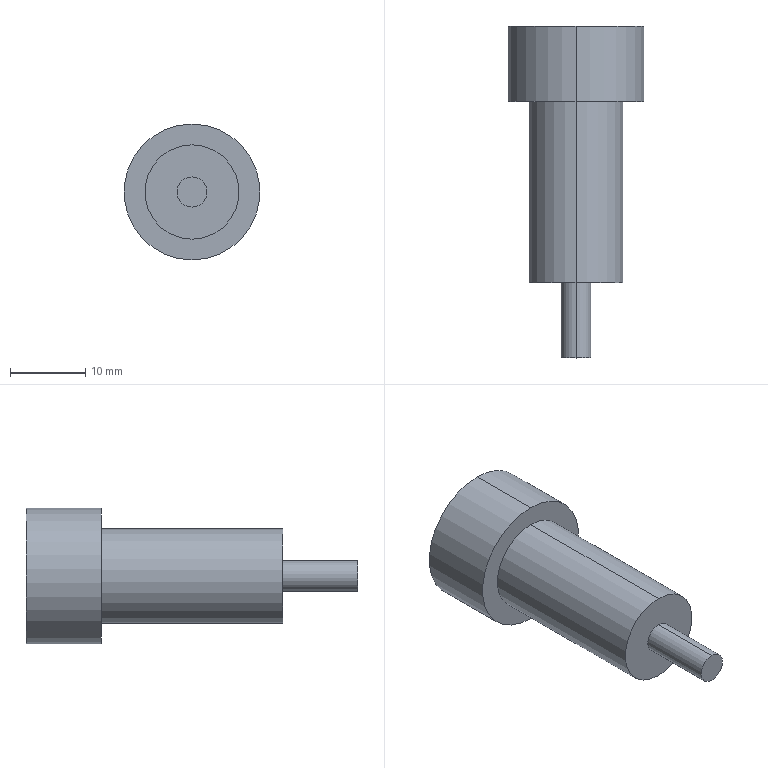Part | SolidWorks | features ICE 3, Extrusion 1 | 1 solid | 17 faces | box 18 x 44 x 18 mm | volume 5338 mm3 | plane 11 | cylinder 6 | commonest cylinder face diameters 4 x2 12.5 x2 18 x2
STEP:
#1=CARTESIAN_POINT('',(0.,44.,9.));
#2=VERTEX_POINT('',#1);
#3=CARTESIAN_POINT('',(0.,44.,-9.));
#4=VERTEX_POINT('',#3);
#5=CARTESIAN_POINT('',(0.,44.,0.));
#6=DIRECTION('',(0.,1.,0.));
#7=DIRECTION('',(0.,0.,1.));
#8=AXIS2_PLACEMENT_3D('',#5,#6,#7);
#9=CIRCLE('',#8,9.);
#10=EDGE_CURVE('',#2,#4,#9,.T.);
#11=ORIENTED_EDGE('',*,*,#10,.F.);
#12=CARTESIAN_POINT('',(0.,34.,9.));
#13=VERTEX_POINT('',#12);
#14=CARTESIAN_POINT('',(0.,44.,9.));
#15=DIRECTION('',(0.,-1.,0.));
#16=VECTOR('',#15,1000.);
#17=LINE('',#14,#16);
#18=EDGE_CURVE('',#2,#13,#17,.T.);
#19=ORIENTED_EDGE('',*,*,#18,.T.);
#20=CARTESIAN_POINT('',(0.,34.,-9.));
#21=VERTEX_POINT('',#20);
#22=CARTESIAN_POINT('',(0.,34.,0.));
#23=DIRECTION('',(0.,1.,0.));
#24=DIRECTION('',(0.,0.,1.));
#25=AXIS2_PLACEMENT_3D('',#22,#23,#24);
#26=CIRCLE('',#25,9.);
#27=EDGE_CURVE('',#13,#21,#26,.T.);
#28=ORIENTED_EDGE('',*,*,#27,.T.);
#29=CARTESIAN_POINT('',(0.,44.,-9.));
#30=DIRECTION('',(0.,-1.,0.));
#31=VECTOR('',#30,1000.);
#32=LINE('',#29,#31);
#33=EDGE_CURVE('',#4,#21,#32,.T.);
#34=ORIENTED_EDGE('',*,*,#33,.F.);
#35=EDGE_LOOP('',(#11,#19,#28,#34));
#36=FACE_OUTER_BOUND('',#35,.T.);
#37=CARTESIAN_POINT('',(0.,44.,0.));
#38=DIRECTION('',(0.,-1.,0.));
#39=DIRECTION('',(0.,0.,-1.));
#40=AXIS2_PLACEMENT_3D('',#37,#38,#39);
#41=CYLINDRICAL_SURFACE('',#40,9.);
#42=ADVANCED_FACE('',(#36),#41,.T.);
#43=CARTESIAN_POINT('',(0.,34.,6.25));
#44=VERTEX_POINT('',#43);
#45=CARTESIAN_POINT('',(0.,34.,-6.25));
#46=VERTEX_POINT('',#45);
#47=CARTESIAN_POINT('',(0.,34.,0.));
#48=DIRECTION('',(0.,1.,0.));
#49=DIRECTION('',(0.,0.,1.));
#50=AXIS2_PLACEMENT_3D('',#47,#48,#49);
#51=CIRCLE('',#50,6.25);
#52=EDGE_CURVE('',#44,#46,#51,.T.);
#53=ORIENTED_EDGE('',*,*,#52,.F.);
#54=CARTESIAN_POINT('',(0.,10.,6.25));
#55=VERTEX_POINT('',#54);
#56=CARTESIAN_POINT('',(0.,34.,6.25));
#57=DIRECTION('',(0.,-1.,0.));
#58=VECTOR('',#57,1000.);
#59=LINE('',#56,#58);
#60=EDGE_CURVE('',#44,#55,#59,.T.);
#61=ORIENTED_EDGE('',*,*,#60,.T.);
#62=CARTESIAN_POINT('',(0.,10.,-6.25));
#63=VERTEX_POINT('',#62);
#64=CARTESIAN_POINT('',(0.,10.,0.));
#65=DIRECTION('',(0.,1.,0.));
#66=DIRECTION('',(0.,0.,1.));
#67=AXIS2_PLACEMENT_3D('',#64,#65,#66);
#68=CIRCLE('',#67,6.25);
#69=EDGE_CURVE('',#55,#63,#68,.T.);
#70=ORIENTED_EDGE('',*,*,#69,.T.);
#71=CARTESIAN_POINT('',(0.,34.,-6.25));
#72=DIRECTION('',(0.,-1.,0.));
#73=VECTOR('',#72,1000.);
#74=LINE('',#71,#73);
#75=EDGE_CURVE('',#46,#63,#74,.T.);
#76=ORIENTED_EDGE('',*,*,#75,.F.);
#77=EDGE_LOOP('',(#53,#61,#70,#76));
#78=FACE_OUTER_BOUND('',#77,.T.);
#79=CARTESIAN_POINT('',(0.,34.,0.));
#80=DIRECTION('',(0.,-1.,0.));
#81=DIRECTION('',(0.,0.,-1.));
#82=AXIS2_PLACEMENT_3D('',#79,#80,#81);
#83=CYLINDRICAL_SURFACE('',#82,6.25);
#84=ADVANCED_FACE('',(#78),#83,.T.);
#85=CARTESIAN_POINT('',(0.,10.,2.));
#86=VERTEX_POINT('',#85);
#87=CARTESIAN_POINT('',(0.,10.,-2.));
#88=VERTEX_POINT('',#87);
#89=CARTESIAN_POINT('',(0.,10.,0.));
#90=DIRECTION('',(0.,1.,0.));
#91=DIRECTION('',(0.,0.,1.));
#92=AXIS2_PLACEMENT_3D('',#89,#90,#91);
#93=CIRCLE('',#92,2.);
#94=EDGE_CURVE('',#86,#88,#93,.T.);
#95=ORIENTED_EDGE('',*,*,#94,.F.);
#96=CARTESIAN_POINT('',(0.,0.,2.));
#97=VERTEX_POINT('',#96);
#98=CARTESIAN_POINT('',(0.,10.,2.));
#99=DIRECTION('',(0.,-1.,0.));
#100=VECTOR('',#99,1000.);
#101=LINE('',#98,#100);
#102=EDGE_CURVE('',#86,#97,#101,.T.);
#103=ORIENTED_EDGE('',*,*,#102,.T.);
#104=CARTESIAN_POINT('',(0.,0.,-2.));
#105=VERTEX_POINT('',#104);
#106=CARTESIAN_POINT('',(0.,0.,0.));
#107=DIRECTION('',(0.,1.,0.));
#108=DIRECTION('',(0.,0.,1.));
#109=AXIS2_PLACEMENT_3D('',#106,#107,#108);
#110=CIRCLE('',#109,2.);
#111=EDGE_CURVE('',#97,#105,#110,.T.);
#112=ORIENTED_EDGE('',*,*,#111,.T.);
#113=CARTESIAN_POINT('',(0.,10.,-2.));
#114=DIRECTION('',(0.,-1.,0.));
#115=VECTOR('',#114,1000.);
#116=LINE('',#113,#115);
#117=EDGE_CURVE('',#88,#105,#116,.T.);
#118=ORIENTED_EDGE('',*,*,#117,.F.);
#119=EDGE_LOOP('',(#95,#103,#112,#118));
#120=FACE_OUTER_BOUND('',#119,.T.);
#121=CARTESIAN_POINT('',(0.,10.,0.));
#122=DIRECTION('',(0.,-1.,0.));
#123=DIRECTION('',(0.,0.,-1.));
#124=AXIS2_PLACEMENT_3D('',#121,#122,#123);
#125=CYLINDRICAL_SURFACE('',#124,2.);
#126=ADVANCED_FACE('',(#120),#125,.T.);
#127=ORIENTED_EDGE('',*,*,#102,.F.);
#128=CARTESIAN_POINT('',(0.,10.,0.));
#129=DIRECTION('',(0.,1.,0.));
#130=DIRECTION('',(0.,0.,1.));
#131=AXIS2_PLACEMENT_3D('',#128,#129,#130);
#132=CIRCLE('',#131,2.);
#133=EDGE_CURVE('',#88,#86,#132,.T.);
#134=ORIENTED_EDGE('',*,*,#133,.F.);
#135=ORIENTED_EDGE('',*,*,#117,.T.);
#136=CARTESIAN_POINT('',(0.,0.,0.));
#137=DIRECTION('',(0.,1.,0.));
#138=DIRECTION('',(0.,0.,1.));
#139=AXIS2_PLACEMENT_3D('',#136,#137,#138);
#140=CIRCLE('',#139,2.);
#141=EDGE_CURVE('',#105,#97,#140,.T.);
#142=ORIENTED_EDGE('',*,*,#141,.T.);
#143=EDGE_LOOP('',(#127,#134,#135,#142));
#144=FACE_OUTER_BOUND('',#143,.T.);
#145=CARTESIAN_POINT('',(0.,10.,0.));
#146=DIRECTION('',(0.,-1.,0.));
#147=DIRECTION('',(0.,0.,-1.));
#148=AXIS2_PLACEMENT_3D('',#145,#146,#147);
#149=CYLINDRICAL_SURFACE('',#148,2.);
#150=ADVANCED_FACE('',(#144),#149,.T.);
#151=ORIENTED_EDGE('',*,*,#141,.F.);
#152=ORIENTED_EDGE('',*,*,#111,.F.);
#153=EDGE_LOOP('',(#151,#152));
#154=FACE_OUTER_BOUND('',#153,.T.);
#155=CARTESIAN_POINT('',(0.,0.,0.));
#156=DIRECTION('',(0.,1.,0.));
#157=DIRECTION('',(0.,0.,1.));
#158=AXIS2_PLACEMENT_3D('',#155,#156,#157);
#159=PLANE('',#158);
#160=ADVANCED_FACE('',(#154),#159,.F.);
#161=ORIENTED_EDGE('',*,*,#60,.F.);
#162=CARTESIAN_POINT('',(0.,34.,0.));
#163=DIRECTION('',(0.,1.,0.));
#164=DIRECTION('',(0.,0.,1.));
#165=AXIS2_PLACEMENT_3D('',#162,#163,#164);
#166=CIRCLE('',#165,6.25);
#167=EDGE_CURVE('',#46,#44,#166,.T.);
#168=ORIENTED_EDGE('',*,*,#167,.F.);
#169=ORIENTED_EDGE('',*,*,#75,.T.);
#170=CARTESIAN_POINT('',(0.,10.,0.));
#171=DIRECTION('',(0.,1.,0.));
#172=DIRECTION('',(0.,0.,1.));
#173=AXIS2_PLACEMENT_3D('',#170,#171,#172);
#174=CIRCLE('',#173,6.25);
#175=EDGE_CURVE('',#63,#55,#174,.T.);
#176=ORIENTED_EDGE('',*,*,#175,.T.);
#177=EDGE_LOOP('',(#161,#168,#169,#176));
#178=FACE_OUTER_BOUND('',#177,.T.);
#179=CARTESIAN_POINT('',(0.,34.,0.));
#180=DIRECTION('',(0.,-1.,0.));
#181=DIRECTION('',(0.,0.,-1.));
#182=AXIS2_PLACEMENT_3D('',#179,#180,#181);
#183=CYLINDRICAL_SURFACE('',#182,6.25);
#184=ADVANCED_FACE('',(#178),#183,.T.);
#185=ORIENTED_EDGE('',*,*,#133,.T.);
#186=ORIENTED_EDGE('',*,*,#94,.T.);
#187=EDGE_LOOP('',(#185,#186));
#188=FACE_BOUND('',#187,.T.);
#189=ORIENTED_EDGE('',*,*,#175,.F.);
#190=ORIENTED_EDGE('',*,*,#69,.F.);
#191=EDGE_LOOP('',(#189,#190));
#192=FACE_OUTER_BOUND('',#191,.T.);
#193=CARTESIAN_POINT('',(0.,10.,0.));
#194=DIRECTION('',(0.,1.,0.));
#195=DIRECTION('',(0.,0.,1.));
#196=AXIS2_PLACEMENT_3D('',#193,#194,#195);
#197=PLANE('',#196);
#198=ADVANCED_FACE('',(#188,#192),#197,.F.);
#199=ORIENTED_EDGE('',*,*,#18,.F.);
#200=CARTESIAN_POINT('',(0.,44.,0.));
#201=DIRECTION('',(0.,1.,0.));
#202=DIRECTION('',(0.,0.,1.));
#203=AXIS2_PLACEMENT_3D('',#200,#201,#202);
#204=CIRCLE('',#203,9.);
#205=EDGE_CURVE('',#4,#2,#204,.T.);
#206=ORIENTED_EDGE('',*,*,#205,.F.);
#207=ORIENTED_EDGE('',*,*,#33,.T.);
#208=CARTESIAN_POINT('',(0.,34.,0.));
#209=DIRECTION('',(0.,1.,0.));
#210=DIRECTION('',(0.,0.,1.));
#211=AXIS2_PLACEMENT_3D('',#208,#209,#210);
#212=CIRCLE('',#211,9.);
#213=EDGE_CURVE('',#21,#13,#212,.T.);
#214=ORIENTED_EDGE('',*,*,#213,.T.);
#215=EDGE_LOOP('',(#199,#206,#207,#214));
#216=FACE_OUTER_BOUND('',#215,.T.);
#217=CARTESIAN_POINT('',(0.,44.,0.));
#218=DIRECTION('',(0.,-1.,0.));
#219=DIRECTION('',(0.,0.,-1.));
#220=AXIS2_PLACEMENT_3D('',#217,#218,#219);
#221=CYLINDRICAL_SURFACE('',#220,9.);
#222=ADVANCED_FACE('',(#216),#221,.T.);
#223=CARTESIAN_POINT('',(4.,44.,-2.309));
#224=VERTEX_POINT('',#223);
#225=CARTESIAN_POINT('',(0.,44.,-4.619));
#226=VERTEX_POINT('',#225);
#227=CARTESIAN_POINT('',(4.,44.,-2.309));
#228=DIRECTION('',(-0.866,0.,-0.5));
#229=VECTOR('',#228,1000.);
#230=LINE('',#227,#229);
#231=EDGE_CURVE('',#224,#226,#230,.T.);
#232=ORIENTED_EDGE('',*,*,#231,.F.);
#233=CARTESIAN_POINT('',(4.,44.,2.309));
#234=VERTEX_POINT('',#233);
#235=CARTESIAN_POINT('',(4.,44.,2.309));
#236=DIRECTION('',(0.,0.,-1.));
#237=VECTOR('',#236,1000.);
#238=LINE('',#235,#237);
#239=EDGE_CURVE('',#234,#224,#238,.T.);
#240=ORIENTED_EDGE('',*,*,#239,.F.);
#241=CARTESIAN_POINT('',(0.,44.,4.619));
#242=VERTEX_POINT('',#241);
#243=CARTESIAN_POINT('',(0.,44.,4.619));
#244=DIRECTION('',(0.866,0.,-0.5));
#245=VECTOR('',#244,1000.);
#246=LINE('',#243,#245);
#247=EDGE_CURVE('',#242,#234,#246,.T.);
#248=ORIENTED_EDGE('',*,*,#247,.F.);
#249=CARTESIAN_POINT('',(-4.,44.,2.309));
#250=VERTEX_POINT('',#249);
#251=CARTESIAN_POINT('',(-4.,44.,2.309));
#252=DIRECTION('',(0.866,0.,0.5));
#253=VECTOR('',#252,1000.);
#254=LINE('',#251,#253);
#255=EDGE_CURVE('',#250,#242,#254,.T.);
#256=ORIENTED_EDGE('',*,*,#255,.F.);
#257=CARTESIAN_POINT('',(-4.,44.,-2.309));
#258=VERTEX_POINT('',#257);
#259=CARTESIAN_POINT('',(-4.,44.,-2.309));
#260=DIRECTION('',(0.,0.,1.));
#261=VECTOR('',#260,1000.);
#262=LINE('',#259,#261);
#263=EDGE_CURVE('',#258,#250,#262,.T.);
#264=ORIENTED_EDGE('',*,*,#263,.F.);
#265=CARTESIAN_POINT('',(0.,44.,-4.619));
#266=DIRECTION('',(-0.866,0.,0.5));
#267=VECTOR('',#266,1000.);
#268=LINE('',#265,#267);
#269=EDGE_CURVE('',#226,#258,#268,.T.);
#270=ORIENTED_EDGE('',*,*,#269,.F.);
#271=EDGE_LOOP('',(#232,#240,#248,#256,#264,#270));
#272=FACE_BOUND('',#271,.T.);
#273=ORIENTED_EDGE('',*,*,#205,.T.);
#274=ORIENTED_EDGE('',*,*,#10,.T.);
#275=EDGE_LOOP('',(#273,#274));
#276=FACE_OUTER_BOUND('',#275,.T.);
#277=CARTESIAN_POINT('',(0.,44.,0.));
#278=DIRECTION('',(0.,1.,0.));
#279=DIRECTION('',(0.,0.,1.));
#280=AXIS2_PLACEMENT_3D('',#277,#278,#279);
#281=PLANE('',#280);
#282=ADVANCED_FACE('',(#272,#276),#281,.T.);
#283=ORIENTED_EDGE('',*,*,#167,.T.);
#284=ORIENTED_EDGE('',*,*,#52,.T.);
#285=EDGE_LOOP('',(#283,#284));
#286=FACE_BOUND('',#285,.T.);
#287=ORIENTED_EDGE('',*,*,#213,.F.);
#288=ORIENTED_EDGE('',*,*,#27,.F.);
#289=EDGE_LOOP('',(#287,#288));
#290=FACE_OUTER_BOUND('',#289,.T.);
#291=CARTESIAN_POINT('',(0.,34.,0.));
#292=DIRECTION('',(0.,1.,0.));
#293=DIRECTION('',(0.,0.,1.));
#294=AXIS2_PLACEMENT_3D('',#291,#292,#293);
#295=PLANE('',#294);
#296=ADVANCED_FACE('',(#286,#290),#295,.F.);
#297=ORIENTED_EDGE('',*,*,#231,.T.);
#298=CARTESIAN_POINT('',(0.,39.,-4.619));
#299=VERTEX_POINT('',#298);
#300=CARTESIAN_POINT('',(0.,39.,-4.619));
#301=DIRECTION('',(0.,1.,0.));
#302=VECTOR('',#301,1000.);
#303=LINE('',#300,#302);
#304=EDGE_CURVE('',#299,#226,#303,.T.);
#305=ORIENTED_EDGE('',*,*,#304,.F.);
#306=CARTESIAN_POINT('',(4.,39.,-2.309));
#307=VERTEX_POINT('',#306);
#308=CARTESIAN_POINT('',(4.,39.,-2.309));
#309=DIRECTION('',(-0.866,0.,-0.5));
#310=VECTOR('',#309,1000.);
#311=LINE('',#308,#310);
#312=EDGE_CURVE('',#307,#299,#311,.T.);
#313=ORIENTED_EDGE('',*,*,#312,.F.);
#314=CARTESIAN_POINT('',(4.,39.,-2.309));
#315=DIRECTION('',(0.,1.,0.));
#316=VECTOR('',#315,1000.);
#317=LINE('',#314,#316);
#318=EDGE_CURVE('',#307,#224,#317,.T.);
#319=ORIENTED_EDGE('',*,*,#318,.T.);
#320=EDGE_LOOP('',(#297,#305,#313,#319));
#321=FACE_OUTER_BOUND('',#320,.T.);
#322=CARTESIAN_POINT('',(4.,39.,-2.309));
#323=DIRECTION('',(0.5,0.,-0.866));
#324=DIRECTION('',(-0.866,0.,-0.5));
#325=AXIS2_PLACEMENT_3D('',#322,#323,#324);
#326=PLANE('',#325);
#327=ADVANCED_FACE('',(#321),#326,.F.);
#328=ORIENTED_EDGE('',*,*,#239,.T.);
#329=ORIENTED_EDGE('',*,*,#318,.F.);
#330=CARTESIAN_POINT('',(4.,39.,2.309));
#331=VERTEX_POINT('',#330);
#332=CARTESIAN_POINT('',(4.,39.,2.309));
#333=DIRECTION('',(0.,0.,-1.));
#334=VECTOR('',#333,1000.);
#335=LINE('',#332,#334);
#336=EDGE_CURVE('',#331,#307,#335,.T.);
#337=ORIENTED_EDGE('',*,*,#336,.F.);
#338=CARTESIAN_POINT('',(4.,39.,2.309));
#339=DIRECTION('',(0.,1.,0.));
#340=VECTOR('',#339,1000.);
#341=LINE('',#338,#340);
#342=EDGE_CURVE('',#331,#234,#341,.T.);
#343=ORIENTED_EDGE('',*,*,#342,.T.);
#344=EDGE_LOOP('',(#328,#329,#337,#343));
#345=FACE_OUTER_BOUND('',#344,.T.);
#346=CARTESIAN_POINT('',(4.,39.,2.309));
#347=DIRECTION('',(1.,0.,0.));
#348=DIRECTION('',(0.,0.,-1.));
#349=AXIS2_PLACEMENT_3D('',#346,#347,#348);
#350=PLANE('',#349);
#351=ADVANCED_FACE('',(#345),#350,.F.);
#352=ORIENTED_EDGE('',*,*,#247,.T.);
#353=ORIENTED_EDGE('',*,*,#342,.F.);
#354=CARTESIAN_POINT('',(0.,39.,4.619));
#355=VERTEX_POINT('',#354);
#356=CARTESIAN_POINT('',(0.,39.,4.619));
#357=DIRECTION('',(0.866,0.,-0.5));
#358=VECTOR('',#357,1000.);
#359=LINE('',#356,#358);
#360=EDGE_CURVE('',#355,#331,#359,.T.);
#361=ORIENTED_EDGE('',*,*,#360,.F.);
#362=CARTESIAN_POINT('',(0.,39.,4.619));
#363=DIRECTION('',(0.,1.,0.));
#364=VECTOR('',#363,1000.);
#365=LINE('',#362,#364);
#366=EDGE_CURVE('',#355,#242,#365,.T.);
#367=ORIENTED_EDGE('',*,*,#366,.T.);
#368=EDGE_LOOP('',(#352,#353,#361,#367));
#369=FACE_OUTER_BOUND('',#368,.T.);
#370=CARTESIAN_POINT('',(0.,39.,4.619));
#371=DIRECTION('',(0.5,0.,0.866));
#372=DIRECTION('',(0.866,0.,-0.5));
#373=AXIS2_PLACEMENT_3D('',#370,#371,#372);
#374=PLANE('',#373);
#375=ADVANCED_FACE('',(#369),#374,.F.);
#376=ORIENTED_EDGE('',*,*,#255,.T.);
#377=ORIENTED_EDGE('',*,*,#366,.F.);
#378=CARTESIAN_POINT('',(-4.,39.,2.309));
#379=VERTEX_POINT('',#378);
#380=CARTESIAN_POINT('',(-4.,39.,2.309));
#381=DIRECTION('',(0.866,0.,0.5));
#382=VECTOR('',#381,1000.);
#383=LINE('',#380,#382);
#384=EDGE_CURVE('',#379,#355,#383,.T.);
#385=ORIENTED_EDGE('',*,*,#384,.F.);
#386=CARTESIAN_POINT('',(-4.,39.,2.309));
#387=DIRECTION('',(0.,1.,0.));
#388=VECTOR('',#387,1000.);
#389=LINE('',#386,#388);
#390=EDGE_CURVE('',#379,#250,#389,.T.);
#391=ORIENTED_EDGE('',*,*,#390,.T.);
#392=EDGE_LOOP('',(#376,#377,#385,#391));
#393=FACE_OUTER_BOUND('',#392,.T.);
#394=CARTESIAN_POINT('',(-4.,39.,2.309));
#395=DIRECTION('',(-0.5,0.,0.866));
#396=DIRECTION('',(0.866,0.,0.5));
#397=AXIS2_PLACEMENT_3D('',#394,#395,#396);
#398=PLANE('',#397);
#399=ADVANCED_FACE('',(#393),#398,.F.);
#400=ORIENTED_EDGE('',*,*,#263,.T.);
#401=ORIENTED_EDGE('',*,*,#390,.F.);
#402=CARTESIAN_POINT('',(-4.,39.,-2.309));
#403=VERTEX_POINT('',#402);
#404=CARTESIAN_POINT('',(-4.,39.,-2.309));
#405=DIRECTION('',(0.,0.,1.));
#406=VECTOR('',#405,1000.);
#407=LINE('',#404,#406);
#408=EDGE_CURVE('',#403,#379,#407,.T.);
#409=ORIENTED_EDGE('',*,*,#408,.F.);
#410=CARTESIAN_POINT('',(-4.,39.,-2.309));
#411=DIRECTION('',(0.,1.,0.));
#412=VECTOR('',#411,1000.);
#413=LINE('',#410,#412);
#414=EDGE_CURVE('',#403,#258,#413,.T.);
#415=ORIENTED_EDGE('',*,*,#414,.T.);
#416=EDGE_LOOP('',(#400,#401,#409,#415));
#417=FACE_OUTER_BOUND('',#416,.T.);
#418=CARTESIAN_POINT('',(-4.,39.,-2.309));
#419=DIRECTION('',(-1.,0.,0.));
#420=DIRECTION('',(0.,0.,1.));
#421=AXIS2_PLACEMENT_3D('',#418,#419,#420);
#422=PLANE('',#421);
#423=ADVANCED_FACE('',(#417),#422,.F.);
#424=ORIENTED_EDGE('',*,*,#269,.T.);
#425=ORIENTED_EDGE('',*,*,#414,.F.);
#426=CARTESIAN_POINT('',(0.,39.,-4.619));
#427=DIRECTION('',(-0.866,0.,0.5));
#428=VECTOR('',#427,1000.);
#429=LINE('',#426,#428);
#430=EDGE_CURVE('',#299,#403,#429,.T.);
#431=ORIENTED_EDGE('',*,*,#430,.F.);
#432=ORIENTED_EDGE('',*,*,#304,.T.);
#433=EDGE_LOOP('',(#424,#425,#431,#432));
#434=FACE_OUTER_BOUND('',#433,.T.);
#435=CARTESIAN_POINT('',(0.,39.,-4.619));
#436=DIRECTION('',(-0.5,0.,-0.866));
#437=DIRECTION('',(-0.866,0.,0.5));
#438=AXIS2_PLACEMENT_3D('',#435,#436,#437);
#439=PLANE('',#438);
#440=ADVANCED_FACE('',(#434),#439,.F.);
#441=ORIENTED_EDGE('',*,*,#312,.T.);
#442=ORIENTED_EDGE('',*,*,#430,.T.);
#443=ORIENTED_EDGE('',*,*,#408,.T.);
#444=ORIENTED_EDGE('',*,*,#384,.T.);
#445=ORIENTED_EDGE('',*,*,#360,.T.);
#446=ORIENTED_EDGE('',*,*,#336,.T.);
#447=EDGE_LOOP('',(#441,#442,#443,#444,#445,#446));
#448=FACE_OUTER_BOUND('',#447,.T.);
#449=CARTESIAN_POINT('',(0.,39.,0.));
#450=DIRECTION('',(0.,1.,0.));
#451=DIRECTION('',(0.,0.,1.));
#452=AXIS2_PLACEMENT_3D('',#449,#450,#451);
#453=PLANE('',#452);
#454=ADVANCED_FACE('',(#448),#453,.T.);
#455=CLOSED_SHELL('',(#42,#84,#126,#150,#160,#184,#198,#222,#282,#296,#327,#351,#375,#399,#423,#440,#454));
#456=MANIFOLD_SOLID_BREP('',#455);
#457=CARTESIAN_POINT('',(0.,0.,0.));
#458=DIRECTION('',(0.,0.,1.));
#459=DIRECTION('',(1.,0.,0.));
#460=AXIS2_PLACEMENT_3D('',#457,#458,#459);
#461=(LENGTH_UNIT()NAMED_UNIT(*)SI_UNIT(.MILLI.,.METRE.));
#462=UNCERTAINTY_MEASURE_WITH_UNIT(LENGTH_MEASURE(0.00001),#461,'','');
#463=(NAMED_UNIT(*)PLANE_ANGLE_UNIT()SI_UNIT($,.RADIAN.));
#464=(NAMED_UNIT(*)SI_UNIT($,.STERADIAN.)SOLID_ANGLE_UNIT());
#465=(GEOMETRIC_REPRESENTATION_CONTEXT(3)GLOBAL_UNCERTAINTY_ASSIGNED_CONTEXT((#462))GLOBAL_UNIT_ASSIGNED_CONTEXT((#461,#463,#464))REPRESENTATION_CONTEXT('',''));
#466=ADVANCED_BREP_SHAPE_REPRESENTATION('',(#456,#460),#465);